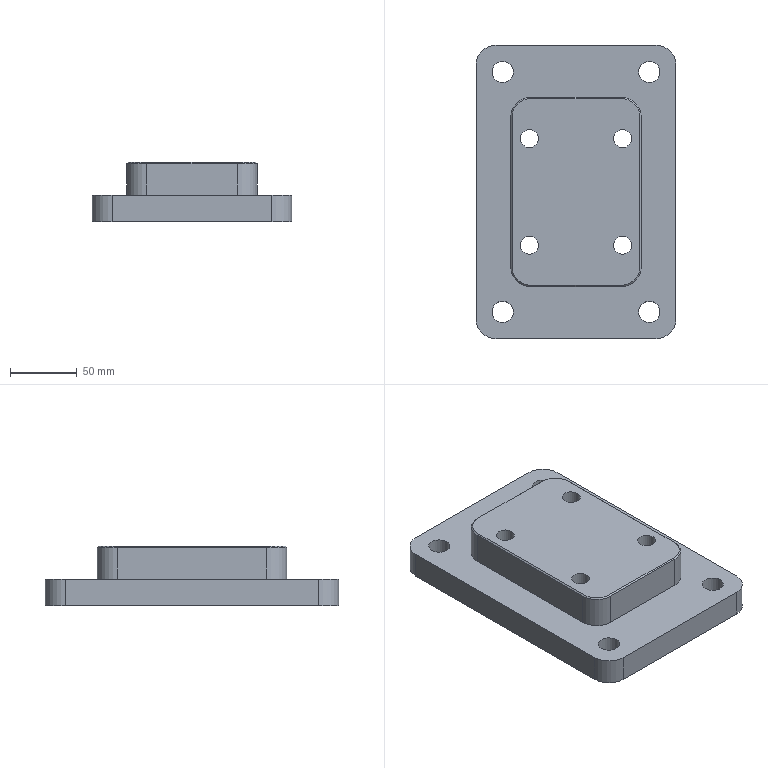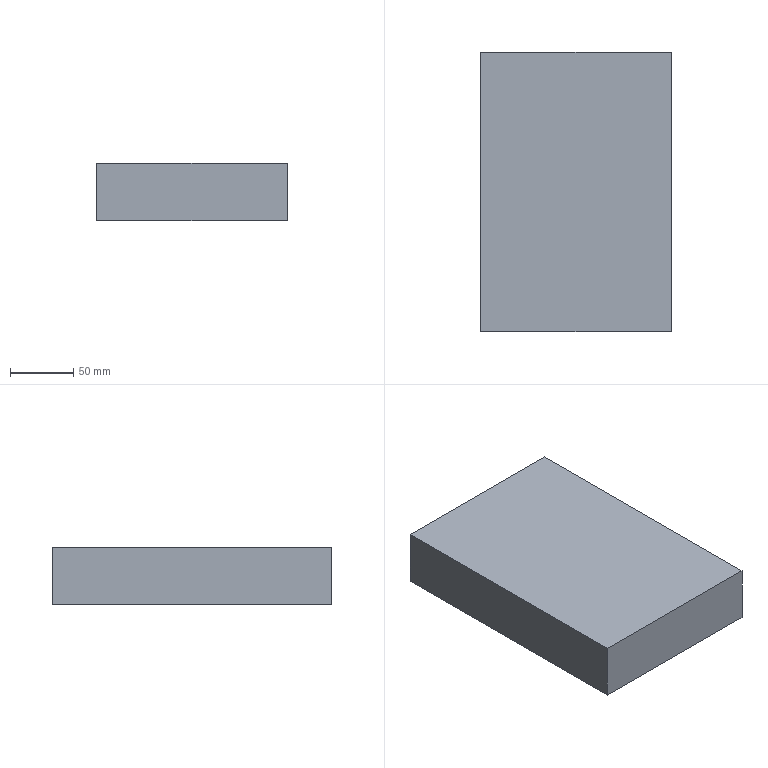CAM job | NX | 3-axis milling, drilling | part box 150 x 220 x 45 mm | stock box 150 x 220 x 45 mm
Tools:
number,name,description,diameter,corner_radius,flute_length,length,flutes
1,ZXZ,Milling Tool-5 Parameters,6.0,0.0,50.0,75.0,2
13,13.5ZT,Drilling Tool,13.5,0.0,35.0,50.0,2
10,D10,Milling Tool-5 Parameters,10.0,0.0,50.0,75.0,2
11,D10JING,Milling Tool-5 Parameters,10.0,0.0,50.0,75.0,2
7,D6A45,Milling Tool-5 Parameters,6.0,0.0,50.0,75.0,2
2,D50,Milling Tool-5 Parameters,50.0,0.0,50.0,75.0,2
Operations:
program,operation,operation_type,tool,method,geometry_group,spindle_rpm,surface_speed,feed_per_tooth,feed_cut,feed_plunge,cut_length_mm,path_length_mm,cut_time_min,machine_time_min
1,DRILLING,Operation,ZXZ,METHOD,A,5000.0,94.0,0.025,250.0,0.0,32.0,630.894,0.128,0.1879
1,DRILLING_COPY,Operation,13.5ZT,METHOD,A,2000.0,84.0,0.05,200.0,0.0,328.447,1223.787,1.642,1.732
1,ZLEVEL_PROFILE_1_COPY,ZLevelMilling,D10,METHOD,A,3200.0,100.0,0.3438,2200.0,100.0,16191.584,44345.105,7.36,10.175
1,HOLE_MILLING,CylinderMilling,D10,METHOD,A,3200.0,100.0,0.3438,2200.0,100.0,19405.67,20519.076,8.821,8.932
1,HOLE_MILLING_COPY,CylinderMilling,D10JING,METHOD,A,5000.0,157.0,0.12,1200.0,100.0,1085.655,2199.062,0.9047,1.016
1,ZLEVEL_PROFILE_1,ZLevelMilling,D10JING,METHOD,A,5000.0,157.0,0.125,1250.0,100.0,207.043,978.294,0.1656,0.2428
1,PLANAR_MILL_COPY_COPY,PlanarMilling,D6A45,METHOD,A,7500.0,141.0,0.0833,1250.0,100.0,1185.451,2208.166,0.9484,1.051
2,ZLEVEL_PROFILE_COPY_COPY,ZLevelMilling,D50,METHOD,B,1200.0,188.0,0.625,1500.0,1000.0,43622.29,43701.14,29.124,29.132
2,FLOOR_WALL,VolumeBased25DMillingOperation,D10JING,METHOD,B,5000.0,157.0,0.12,1200.0,500.0,4719.972,5549.23,3.802,3.885
2,PLANAR_MILL_COPY_COPY_COPY,PlanarMilling,D6A45,METHOD,B,7500.0,141.0,0.0833,1250.0,100.0,181.005,648.007,0.1448,0.1915
2,PLANAR_MILL_COPY_COPY_COPY_COPY,PlanarMilling,D6A45,METHOD,B,7500.0,141.0,0.0833,1250.0,100.0,470.477,528.477,0.3764,0.3822
2,PLANAR_MILL_COPY_COPY_COPY_COPY_1,PlanarMilling,D6A45,METHOD,B,7500.0,141.0,0.0833,1250.0,100.0,929.532,1886.579,0.7436,0.8393